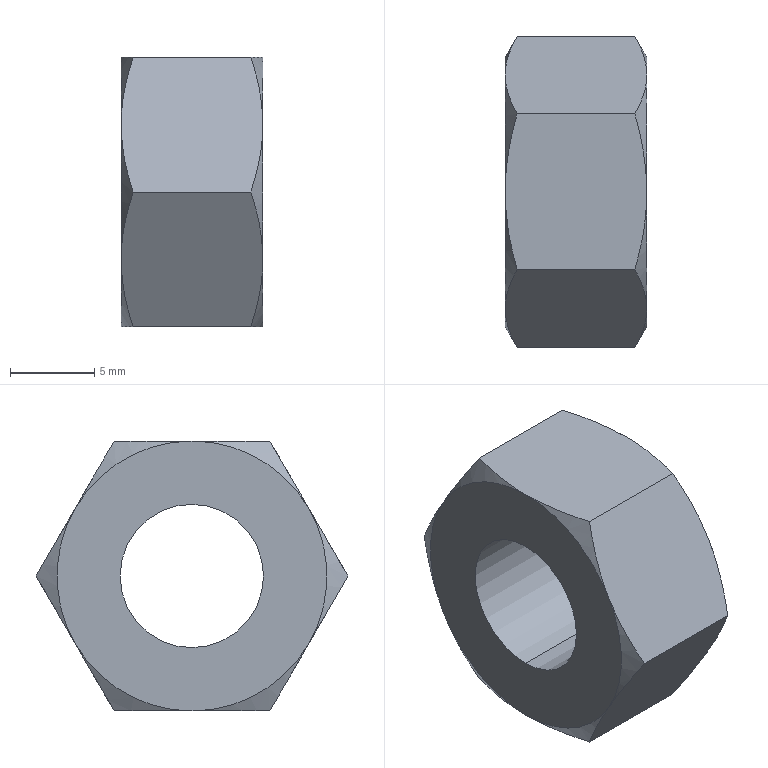Part | SolidWorks | features 3DProfileFeature 1, Extrusion 1, HoleWzd 1, ICE 1, MirrorPattern 1, RevCut 1 | 1 solid | 68 faces | box 8.4 x 18.475 x 16 mm | volume 1377 mm3 | plane 36 | spline 18 | cone 12 | cylinder 2 | commonest cylinder face diameters 8.5 x2